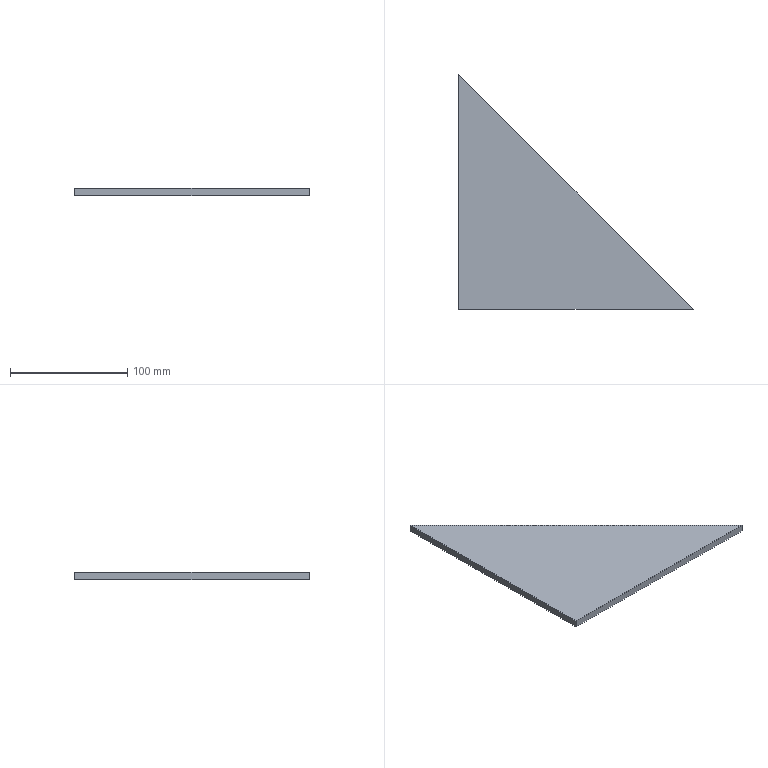Part | STEP file | BCC3 H13_9B | 1 solid | 5 faces | box 200 x 200 x 6 mm | volume 120000 mm3 | plane 5
STEP:
#1=CARTESIAN_POINT('',(0.,0.,0.));
#2=DIRECTION('',(0.,0.,1.));
#3=DIRECTION('',(1.,0.,0.));
#4=AXIS2_PLACEMENT_3D('',#1,#2,#3);
#5=CARTESIAN_POINT('',(0.,0.,-3.));
#6=VERTEX_POINT('',#5);
#7=CARTESIAN_POINT('',(200.,0.,-3.));
#8=VERTEX_POINT('',#7);
#9=CARTESIAN_POINT('',(200.,0.,-3.));
#10=DIRECTION('',(1.,0.,0.));
#11=VECTOR('',#10,1.);
#12=LINE('',#9,#11);
#13=CARTESIAN_POINT('',(200.,0.,3.));
#14=DIRECTION('',(0.,1.,0.));
#15=DIRECTION('',(-1.,0.,0.));
#16=AXIS2_PLACEMENT_3D('',#13,#14,#15);
#17=PLANE('',#16);
#18=CARTESIAN_POINT('',(0.,-6.));
#19=DIRECTION('',(-1.,0.));
#20=VECTOR('',#19,1.);
#21=LINE('',#18,#20);
#22=(GEOMETRIC_REPRESENTATION_CONTEXT(2)PARAMETRIC_REPRESENTATION_CONTEXT()REPRESENTATION_CONTEXT('',''));
#23=DEFINITIONAL_REPRESENTATION('',(#21),#22);
#24=PCURVE('',#17,#23);
#25=CARTESIAN_POINT('',(0.,0.,-3.));
#26=DIRECTION('',(0.,0.,-1.));
#27=DIRECTION('',(-1.,0.,0.));
#28=AXIS2_PLACEMENT_3D('',#25,#26,#27);
#29=PLANE('',#28);
#30=CARTESIAN_POINT('',(-200.,0.));
#31=DIRECTION('',(-1.,0.));
#32=VECTOR('',#31,1.);
#33=LINE('',#30,#32);
#34=(GEOMETRIC_REPRESENTATION_CONTEXT(2)PARAMETRIC_REPRESENTATION_CONTEXT()REPRESENTATION_CONTEXT('',''));
#35=DEFINITIONAL_REPRESENTATION('',(#33),#34);
#36=PCURVE('',#29,#35);
#37=SURFACE_CURVE('',#12,(#24,#36),.PCURVE_S1.);
#38=EDGE_CURVE('',#6,#8,#37,.T.);
#39=ORIENTED_EDGE('',*,*,#38,.T.);
#40=CARTESIAN_POINT('',(200.,0.,3.));
#41=VERTEX_POINT('',#40);
#42=CARTESIAN_POINT('',(200.,0.,3.));
#43=DIRECTION('',(0.,0.,-1.));
#44=VECTOR('',#43,1.);
#45=LINE('',#42,#44);
#46=CARTESIAN_POINT('',(0.,0.));
#47=DIRECTION('',(0.,-1.));
#48=VECTOR('',#47,1.);
#49=LINE('',#46,#48);
#50=(GEOMETRIC_REPRESENTATION_CONTEXT(2)PARAMETRIC_REPRESENTATION_CONTEXT()REPRESENTATION_CONTEXT('',''));
#51=DEFINITIONAL_REPRESENTATION('',(#49),#50);
#52=PCURVE('',#17,#51);
#53=CARTESIAN_POINT('',(0.,200.,3.));
#54=DIRECTION('',(-0.7071,-0.7071,0.));
#55=DIRECTION('',(0.7071,-0.7071,0.));
#56=AXIS2_PLACEMENT_3D('',#53,#54,#55);
#57=PLANE('',#56);
#58=CARTESIAN_POINT('',(282.843,0.));
#59=DIRECTION('',(0.,-1.));
#60=VECTOR('',#59,1.);
#61=LINE('',#58,#60);
#62=(GEOMETRIC_REPRESENTATION_CONTEXT(2)PARAMETRIC_REPRESENTATION_CONTEXT()REPRESENTATION_CONTEXT('',''));
#63=DEFINITIONAL_REPRESENTATION('',(#61),#62);
#64=PCURVE('',#57,#63);
#65=SURFACE_CURVE('',#45,(#52,#64),.PCURVE_S1.);
#66=EDGE_CURVE('',#41,#8,#65,.T.);
#67=ORIENTED_EDGE('',*,*,#66,.F.);
#68=CARTESIAN_POINT('',(0.,0.,3.));
#69=VERTEX_POINT('',#68);
#70=CARTESIAN_POINT('',(200.,0.,3.));
#71=DIRECTION('',(1.,0.,0.));
#72=VECTOR('',#71,1.);
#73=LINE('',#70,#72);
#74=CARTESIAN_POINT('',(0.,0.));
#75=DIRECTION('',(-1.,0.));
#76=VECTOR('',#75,1.);
#77=LINE('',#74,#76);
#78=(GEOMETRIC_REPRESENTATION_CONTEXT(2)PARAMETRIC_REPRESENTATION_CONTEXT()REPRESENTATION_CONTEXT('',''));
#79=DEFINITIONAL_REPRESENTATION('',(#77),#78);
#80=PCURVE('',#17,#79);
#81=CARTESIAN_POINT('',(0.,0.,3.));
#82=DIRECTION('',(0.,0.,-1.));
#83=DIRECTION('',(-1.,0.,0.));
#84=AXIS2_PLACEMENT_3D('',#81,#82,#83);
#85=PLANE('',#84);
#86=CARTESIAN_POINT('',(-200.,0.));
#87=DIRECTION('',(-1.,0.));
#88=VECTOR('',#87,1.);
#89=LINE('',#86,#88);
#90=(GEOMETRIC_REPRESENTATION_CONTEXT(2)PARAMETRIC_REPRESENTATION_CONTEXT()REPRESENTATION_CONTEXT('',''));
#91=DEFINITIONAL_REPRESENTATION('',(#89),#90);
#92=PCURVE('',#85,#91);
#93=SURFACE_CURVE('',#73,(#80,#92),.PCURVE_S1.);
#94=EDGE_CURVE('',#69,#41,#93,.T.);
#95=ORIENTED_EDGE('',*,*,#94,.F.);
#96=CARTESIAN_POINT('',(0.,0.,3.));
#97=DIRECTION('',(0.,0.,-1.));
#98=VECTOR('',#97,1.);
#99=LINE('',#96,#98);
#100=CARTESIAN_POINT('',(200.,0.));
#101=DIRECTION('',(0.,-1.));
#102=VECTOR('',#101,1.);
#103=LINE('',#100,#102);
#104=(GEOMETRIC_REPRESENTATION_CONTEXT(2)PARAMETRIC_REPRESENTATION_CONTEXT()REPRESENTATION_CONTEXT('',''));
#105=DEFINITIONAL_REPRESENTATION('',(#103),#104);
#106=PCURVE('',#17,#105);
#107=CARTESIAN_POINT('',(0.,0.,3.));
#108=DIRECTION('',(1.,0.,0.));
#109=DIRECTION('',(0.,0.,-1.));
#110=AXIS2_PLACEMENT_3D('',#107,#108,#109);
#111=PLANE('',#110);
#112=CARTESIAN_POINT('',(0.,0.));
#113=DIRECTION('',(1.,0.));
#114=VECTOR('',#113,1.);
#115=LINE('',#112,#114);
#116=(GEOMETRIC_REPRESENTATION_CONTEXT(2)PARAMETRIC_REPRESENTATION_CONTEXT()REPRESENTATION_CONTEXT('',''));
#117=DEFINITIONAL_REPRESENTATION('',(#115),#116);
#118=PCURVE('',#111,#117);
#119=SURFACE_CURVE('',#99,(#106,#118),.PCURVE_S1.);
#120=EDGE_CURVE('',#69,#6,#119,.T.);
#121=ORIENTED_EDGE('',*,*,#120,.T.);
#122=EDGE_LOOP('',(#39,#67,#95,#121));
#123=FACE_BOUND('',#122,.T.);
#124=ADVANCED_FACE('',(#123),#17,.F.);
#125=CARTESIAN_POINT('',(0.,200.,-3.));
#126=VERTEX_POINT('',#125);
#127=CARTESIAN_POINT('',(0.,200.,-3.));
#128=DIRECTION('',(-0.7071,0.7071,0.));
#129=VECTOR('',#128,1.);
#130=LINE('',#127,#129);
#131=CARTESIAN_POINT('',(0.,-6.));
#132=DIRECTION('',(-1.,0.));
#133=VECTOR('',#132,1.);
#134=LINE('',#131,#133);
#135=(GEOMETRIC_REPRESENTATION_CONTEXT(2)PARAMETRIC_REPRESENTATION_CONTEXT()REPRESENTATION_CONTEXT('',''));
#136=DEFINITIONAL_REPRESENTATION('',(#134),#135);
#137=PCURVE('',#57,#136);
#138=CARTESIAN_POINT('',(0.,200.));
#139=DIRECTION('',(0.7071,0.7071));
#140=VECTOR('',#139,1.);
#141=LINE('',#138,#140);
#142=(GEOMETRIC_REPRESENTATION_CONTEXT(2)PARAMETRIC_REPRESENTATION_CONTEXT()REPRESENTATION_CONTEXT('',''));
#143=DEFINITIONAL_REPRESENTATION('',(#141),#142);
#144=PCURVE('',#29,#143);
#145=SURFACE_CURVE('',#130,(#137,#144),.PCURVE_S1.);
#146=EDGE_CURVE('',#8,#126,#145,.T.);
#147=ORIENTED_EDGE('',*,*,#146,.T.);
#148=CARTESIAN_POINT('',(0.,200.,3.));
#149=VERTEX_POINT('',#148);
#150=CARTESIAN_POINT('',(0.,200.,3.));
#151=DIRECTION('',(0.,0.,-1.));
#152=VECTOR('',#151,1.);
#153=LINE('',#150,#152);
#154=CARTESIAN_POINT('',(0.,0.));
#155=DIRECTION('',(0.,-1.));
#156=VECTOR('',#155,1.);
#157=LINE('',#154,#156);
#158=(GEOMETRIC_REPRESENTATION_CONTEXT(2)PARAMETRIC_REPRESENTATION_CONTEXT()REPRESENTATION_CONTEXT('',''));
#159=DEFINITIONAL_REPRESENTATION('',(#157),#158);
#160=PCURVE('',#57,#159);
#161=CARTESIAN_POINT('',(0.,200.));
#162=DIRECTION('',(1.,0.));
#163=VECTOR('',#162,1.);
#164=LINE('',#161,#163);
#165=(GEOMETRIC_REPRESENTATION_CONTEXT(2)PARAMETRIC_REPRESENTATION_CONTEXT()REPRESENTATION_CONTEXT('',''));
#166=DEFINITIONAL_REPRESENTATION('',(#164),#165);
#167=PCURVE('',#111,#166);
#168=SURFACE_CURVE('',#153,(#160,#167),.PCURVE_S1.);
#169=EDGE_CURVE('',#149,#126,#168,.T.);
#170=ORIENTED_EDGE('',*,*,#169,.F.);
#171=CARTESIAN_POINT('',(0.,200.,3.));
#172=DIRECTION('',(-0.7071,0.7071,0.));
#173=VECTOR('',#172,1.);
#174=LINE('',#171,#173);
#175=CARTESIAN_POINT('',(0.,0.));
#176=DIRECTION('',(-1.,0.));
#177=VECTOR('',#176,1.);
#178=LINE('',#175,#177);
#179=(GEOMETRIC_REPRESENTATION_CONTEXT(2)PARAMETRIC_REPRESENTATION_CONTEXT()REPRESENTATION_CONTEXT('',''));
#180=DEFINITIONAL_REPRESENTATION('',(#178),#179);
#181=PCURVE('',#57,#180);
#182=CARTESIAN_POINT('',(0.,200.));
#183=DIRECTION('',(0.7071,0.7071));
#184=VECTOR('',#183,1.);
#185=LINE('',#182,#184);
#186=(GEOMETRIC_REPRESENTATION_CONTEXT(2)PARAMETRIC_REPRESENTATION_CONTEXT()REPRESENTATION_CONTEXT('',''));
#187=DEFINITIONAL_REPRESENTATION('',(#185),#186);
#188=PCURVE('',#85,#187);
#189=SURFACE_CURVE('',#174,(#181,#188),.PCURVE_S1.);
#190=EDGE_CURVE('',#41,#149,#189,.T.);
#191=ORIENTED_EDGE('',*,*,#190,.F.);
#192=ORIENTED_EDGE('',*,*,#66,.T.);
#193=EDGE_LOOP('',(#147,#170,#191,#192));
#194=FACE_BOUND('',#193,.T.);
#195=ADVANCED_FACE('',(#194),#57,.F.);
#196=CARTESIAN_POINT('',(0.,0.,-3.));
#197=DIRECTION('',(0.,-1.,0.));
#198=VECTOR('',#197,1.);
#199=LINE('',#196,#198);
#200=CARTESIAN_POINT('',(6.,0.));
#201=DIRECTION('',(0.,-1.));
#202=VECTOR('',#201,1.);
#203=LINE('',#200,#202);
#204=(GEOMETRIC_REPRESENTATION_CONTEXT(2)PARAMETRIC_REPRESENTATION_CONTEXT()REPRESENTATION_CONTEXT('',''));
#205=DEFINITIONAL_REPRESENTATION('',(#203),#204);
#206=PCURVE('',#111,#205);
#207=CARTESIAN_POINT('',(0.,0.));
#208=DIRECTION('',(0.,-1.));
#209=VECTOR('',#208,1.);
#210=LINE('',#207,#209);
#211=(GEOMETRIC_REPRESENTATION_CONTEXT(2)PARAMETRIC_REPRESENTATION_CONTEXT()REPRESENTATION_CONTEXT('',''));
#212=DEFINITIONAL_REPRESENTATION('',(#210),#211);
#213=PCURVE('',#29,#212);
#214=SURFACE_CURVE('',#199,(#206,#213),.PCURVE_S1.);
#215=EDGE_CURVE('',#126,#6,#214,.T.);
#216=ORIENTED_EDGE('',*,*,#215,.T.);
#217=ORIENTED_EDGE('',*,*,#120,.F.);
#218=CARTESIAN_POINT('',(0.,0.,3.));
#219=DIRECTION('',(0.,-1.,0.));
#220=VECTOR('',#219,1.);
#221=LINE('',#218,#220);
#222=CARTESIAN_POINT('',(0.,0.));
#223=DIRECTION('',(0.,-1.));
#224=VECTOR('',#223,1.);
#225=LINE('',#222,#224);
#226=(GEOMETRIC_REPRESENTATION_CONTEXT(2)PARAMETRIC_REPRESENTATION_CONTEXT()REPRESENTATION_CONTEXT('',''));
#227=DEFINITIONAL_REPRESENTATION('',(#225),#226);
#228=PCURVE('',#111,#227);
#229=CARTESIAN_POINT('',(0.,0.));
#230=DIRECTION('',(0.,-1.));
#231=VECTOR('',#230,1.);
#232=LINE('',#229,#231);
#233=(GEOMETRIC_REPRESENTATION_CONTEXT(2)PARAMETRIC_REPRESENTATION_CONTEXT()REPRESENTATION_CONTEXT('',''));
#234=DEFINITIONAL_REPRESENTATION('',(#232),#233);
#235=PCURVE('',#85,#234);
#236=SURFACE_CURVE('',#221,(#228,#235),.PCURVE_S1.);
#237=EDGE_CURVE('',#149,#69,#236,.T.);
#238=ORIENTED_EDGE('',*,*,#237,.F.);
#239=ORIENTED_EDGE('',*,*,#169,.T.);
#240=EDGE_LOOP('',(#216,#217,#238,#239));
#241=FACE_BOUND('',#240,.T.);
#242=ADVANCED_FACE('',(#241),#111,.F.);
#243=ORIENTED_EDGE('',*,*,#94,.T.);
#244=ORIENTED_EDGE('',*,*,#190,.T.);
#245=ORIENTED_EDGE('',*,*,#237,.T.);
#246=EDGE_LOOP('',(#243,#244,#245));
#247=FACE_BOUND('',#246,.T.);
#248=ADVANCED_FACE('',(#247),#85,.F.);
#249=ORIENTED_EDGE('',*,*,#38,.F.);
#250=ORIENTED_EDGE('',*,*,#215,.F.);
#251=ORIENTED_EDGE('',*,*,#146,.F.);
#252=EDGE_LOOP('',(#249,#250,#251));
#253=FACE_BOUND('',#252,.T.);
#254=ADVANCED_FACE('',(#253),#29,.T.);
#255=CLOSED_SHELL('',(#124,#195,#242,#248,#254));
#256=MANIFOLD_SOLID_BREP('',#255);
#257=(LENGTH_UNIT()NAMED_UNIT(*)SI_UNIT(.MILLI.,.METRE.));
#258=UNCERTAINTY_MEASURE_WITH_UNIT(LENGTH_MEASURE(0.0000001),#257,'','');
#259=(NAMED_UNIT(*)PLANE_ANGLE_UNIT()SI_UNIT($,.RADIAN.));
#260=(NAMED_UNIT(*)SI_UNIT($,.STERADIAN.)SOLID_ANGLE_UNIT());
#261=(GEOMETRIC_REPRESENTATION_CONTEXT(3)GLOBAL_UNCERTAINTY_ASSIGNED_CONTEXT((#258))GLOBAL_UNIT_ASSIGNED_CONTEXT((#257,#259,#260))REPRESENTATION_CONTEXT('',''));
#262=ADVANCED_BREP_SHAPE_REPRESENTATION('',(#4,#256),#261);